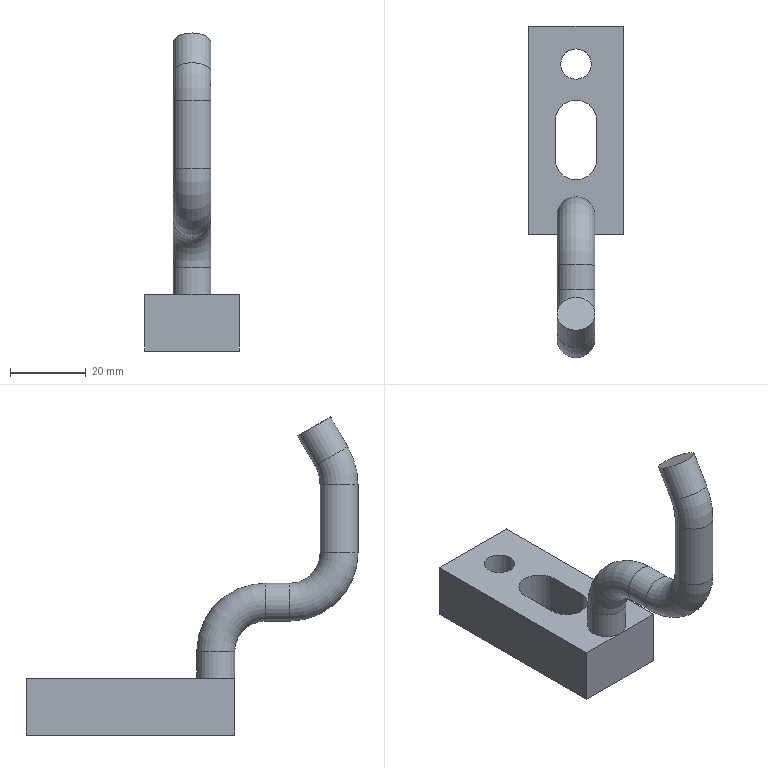Part | NX | features solid 2 | 1 solid | 19 faces | box 25 x 87.5 x 83.84 mm | volume 23805 mm3 | plane 9 | cylinder 7 | torus 3 | commonest cylinder face diameters 10 x4 11 x2 8 x1
STEP:
#1=CARTESIAN_POINT('',(-37.5,251.,-40.));
#2=VERTEX_POINT('',#1);
#3=CARTESIAN_POINT('',(-25.,251.,-40.));
#4=VERTEX_POINT('',#3);
#5=CARTESIAN_POINT('',(-37.,251.,-40.));
#6=DIRECTION('',(-1.,0.,0.));
#7=VECTOR('',#6,1000.);
#8=LINE('',#5,#7);
#9=EDGE_CURVE('',#2,#4,#8,.F.);
#10=ORIENTED_EDGE('',*,*,#9,.T.);
#11=CARTESIAN_POINT('',(-25.,256.,-40.));
#12=DIRECTION('',(0.,0.,1.));
#13=DIRECTION('',(0.,-1.,0.));
#14=AXIS2_PLACEMENT_3D('',#11,#12,#13);
#15=CIRCLE('',#14,5.);
#16=EDGE_CURVE('',#4,#4,#15,.T.);
#17=ORIENTED_EDGE('',*,*,#16,.F.);
#18=CARTESIAN_POINT('',(-12.5,251.,-40.));
#19=VERTEX_POINT('',#18);
#20=CARTESIAN_POINT('',(-37.,251.,-40.));
#21=DIRECTION('',(-1.,0.,0.));
#22=VECTOR('',#21,1000.);
#23=LINE('',#20,#22);
#24=EDGE_CURVE('',#4,#19,#23,.F.);
#25=ORIENTED_EDGE('',*,*,#24,.T.);
#26=CARTESIAN_POINT('',(-12.5,306.,-40.));
#27=VERTEX_POINT('',#26);
#28=CARTESIAN_POINT('',(-12.5,251.,-40.));
#29=DIRECTION('',(0.,1.,0.));
#30=VECTOR('',#29,1000.);
#31=LINE('',#28,#30);
#32=EDGE_CURVE('',#19,#27,#31,.T.);
#33=ORIENTED_EDGE('',*,*,#32,.T.);
#34=CARTESIAN_POINT('',(-37.5,306.,-40.));
#35=VERTEX_POINT('',#34);
#36=CARTESIAN_POINT('',(-37.,306.,-40.));
#37=DIRECTION('',(-1.,0.,0.));
#38=VECTOR('',#37,1000.);
#39=LINE('',#36,#38);
#40=EDGE_CURVE('',#27,#35,#39,.T.);
#41=ORIENTED_EDGE('',*,*,#40,.T.);
#42=CARTESIAN_POINT('',(-37.5,321.,-40.));
#43=DIRECTION('',(0.,-1.,0.));
#44=VECTOR('',#43,1000.);
#45=LINE('',#42,#44);
#46=EDGE_CURVE('',#35,#2,#45,.T.);
#47=ORIENTED_EDGE('',*,*,#46,.T.);
#48=EDGE_LOOP('',(#10,#17,#25,#33,#41,#47));
#49=FACE_BOUND('',#48,.T.);
#50=CARTESIAN_POINT('',(-30.5,271.,-40.));
#51=VERTEX_POINT('',#50);
#52=CARTESIAN_POINT('',(-30.5,281.,-40.));
#53=VERTEX_POINT('',#52);
#54=CARTESIAN_POINT('',(-30.5,281.,-40.));
#55=DIRECTION('',(0.,1.,0.));
#56=VECTOR('',#55,1000.);
#57=LINE('',#54,#56);
#58=EDGE_CURVE('',#51,#53,#57,.T.);
#59=ORIENTED_EDGE('',*,*,#58,.T.);
#60=CARTESIAN_POINT('',(-19.5,281.,-40.));
#61=VERTEX_POINT('',#60);
#62=CARTESIAN_POINT('',(-25.,281.,-40.));
#63=DIRECTION('',(0.,0.,1.));
#64=DIRECTION('',(0.,1.,0.));
#65=AXIS2_PLACEMENT_3D('',#62,#63,#64);
#66=CIRCLE('',#65,5.5);
#67=EDGE_CURVE('',#61,#53,#66,.T.);
#68=ORIENTED_EDGE('',*,*,#67,.F.);
#69=CARTESIAN_POINT('',(-19.5,271.,-40.));
#70=VERTEX_POINT('',#69);
#71=CARTESIAN_POINT('',(-19.5,286.,-40.));
#72=DIRECTION('',(0.,1.,0.));
#73=VECTOR('',#72,1000.);
#74=LINE('',#71,#73);
#75=EDGE_CURVE('',#70,#61,#74,.T.);
#76=ORIENTED_EDGE('',*,*,#75,.F.);
#77=CARTESIAN_POINT('',(-25.,271.,-40.));
#78=DIRECTION('',(0.,0.,1.));
#79=DIRECTION('',(0.,1.,0.));
#80=AXIS2_PLACEMENT_3D('',#77,#78,#79);
#81=CIRCLE('',#80,5.5);
#82=EDGE_CURVE('',#51,#70,#81,.T.);
#83=ORIENTED_EDGE('',*,*,#82,.F.);
#84=EDGE_LOOP('',(#59,#68,#76,#83));
#85=FACE_BOUND('',#84,.T.);
#86=CARTESIAN_POINT('',(-25.,292.,-40.));
#87=VERTEX_POINT('',#86);
#88=CARTESIAN_POINT('',(-25.,296.,-40.));
#89=DIRECTION('',(0.,0.,-1.));
#90=DIRECTION('',(0.,-1.,0.));
#91=AXIS2_PLACEMENT_3D('',#88,#89,#90);
#92=CIRCLE('',#91,4.);
#93=EDGE_CURVE('',#87,#87,#92,.T.);
#94=ORIENTED_EDGE('',*,*,#93,.T.);
#95=EDGE_LOOP('',(#94));
#96=FACE_BOUND('',#95,.T.);
#97=CARTESIAN_POINT('',(-37.,321.,-40.));
#98=DIRECTION('',(0.,0.,1.));
#99=DIRECTION('',(0.,-1.,0.));
#100=AXIS2_PLACEMENT_3D('',#97,#98,#99);
#101=PLANE('',#100);
#102=ADVANCED_FACE('',(#49,#85,#96),#101,.T.);
#103=CARTESIAN_POINT('',(-37.5,306.,-55.));
#104=VERTEX_POINT('',#103);
#105=CARTESIAN_POINT('',(-37.5,251.,-55.));
#106=VERTEX_POINT('',#105);
#107=CARTESIAN_POINT('',(-37.5,321.,-55.));
#108=DIRECTION('',(0.,-1.,0.));
#109=VECTOR('',#108,1000.);
#110=LINE('',#107,#109);
#111=EDGE_CURVE('',#104,#106,#110,.T.);
#112=ORIENTED_EDGE('',*,*,#111,.T.);
#113=CARTESIAN_POINT('',(-37.5,251.,-65.));
#114=DIRECTION('',(0.,0.,-1.));
#115=VECTOR('',#114,1000.);
#116=LINE('',#113,#115);
#117=EDGE_CURVE('',#2,#106,#116,.T.);
#118=ORIENTED_EDGE('',*,*,#117,.F.);
#119=ORIENTED_EDGE('',*,*,#46,.F.);
#120=CARTESIAN_POINT('',(-37.5,306.,-65.));
#121=DIRECTION('',(0.,0.,-1.));
#122=VECTOR('',#121,1000.);
#123=LINE('',#120,#122);
#124=EDGE_CURVE('',#35,#104,#123,.T.);
#125=ORIENTED_EDGE('',*,*,#124,.T.);
#126=EDGE_LOOP('',(#112,#118,#119,#125));
#127=FACE_BOUND('',#126,.T.);
#128=CARTESIAN_POINT('',(-37.5,321.,-65.));
#129=DIRECTION('',(1.,0.,0.));
#130=DIRECTION('',(0.,1.,0.));
#131=AXIS2_PLACEMENT_3D('',#128,#129,#130);
#132=PLANE('',#131);
#133=ADVANCED_FACE('',(#127),#132,.F.);
#134=CARTESIAN_POINT('',(-12.5,306.,-55.));
#135=VERTEX_POINT('',#134);
#136=CARTESIAN_POINT('',(-37.,306.,-55.));
#137=DIRECTION('',(-1.,0.,0.));
#138=VECTOR('',#137,1000.);
#139=LINE('',#136,#138);
#140=EDGE_CURVE('',#135,#104,#139,.T.);
#141=ORIENTED_EDGE('',*,*,#140,.T.);
#142=ORIENTED_EDGE('',*,*,#124,.F.);
#143=ORIENTED_EDGE('',*,*,#40,.F.);
#144=CARTESIAN_POINT('',(-12.5,306.,-40.));
#145=DIRECTION('',(0.,0.,-1.));
#146=VECTOR('',#145,1000.);
#147=LINE('',#144,#146);
#148=EDGE_CURVE('',#27,#135,#147,.T.);
#149=ORIENTED_EDGE('',*,*,#148,.T.);
#150=EDGE_LOOP('',(#141,#142,#143,#149));
#151=FACE_BOUND('',#150,.T.);
#152=CARTESIAN_POINT('',(-13.,306.,-65.));
#153=DIRECTION('',(0.,-1.,0.));
#154=DIRECTION('',(0.,0.,1.));
#155=AXIS2_PLACEMENT_3D('',#152,#153,#154);
#156=PLANE('',#155);
#157=ADVANCED_FACE('',(#151),#156,.F.);
#158=CARTESIAN_POINT('',(-12.5,251.,-55.));
#159=VERTEX_POINT('',#158);
#160=CARTESIAN_POINT('',(-12.5,321.,-55.));
#161=DIRECTION('',(0.,1.,0.));
#162=VECTOR('',#161,1000.);
#163=LINE('',#160,#162);
#164=EDGE_CURVE('',#159,#135,#163,.T.);
#165=ORIENTED_EDGE('',*,*,#164,.T.);
#166=ORIENTED_EDGE('',*,*,#148,.F.);
#167=ORIENTED_EDGE('',*,*,#32,.F.);
#168=CARTESIAN_POINT('',(-12.5,251.,-40.));
#169=DIRECTION('',(0.,0.,-1.));
#170=VECTOR('',#169,1000.);
#171=LINE('',#168,#170);
#172=EDGE_CURVE('',#19,#159,#171,.T.);
#173=ORIENTED_EDGE('',*,*,#172,.T.);
#174=EDGE_LOOP('',(#165,#166,#167,#173));
#175=FACE_BOUND('',#174,.T.);
#176=CARTESIAN_POINT('',(-12.5,251.,-40.));
#177=DIRECTION('',(-1.,0.,0.));
#178=DIRECTION('',(0.,-1.,0.));
#179=AXIS2_PLACEMENT_3D('',#176,#177,#178);
#180=PLANE('',#179);
#181=ADVANCED_FACE('',(#175),#180,.F.);
#182=ORIENTED_EDGE('',*,*,#93,.F.);
#183=EDGE_LOOP('',(#182));
#184=FACE_BOUND('',#183,.T.);
#185=CARTESIAN_POINT('',(-25.,292.,-55.));
#186=VERTEX_POINT('',#185);
#187=CARTESIAN_POINT('',(-25.,296.,-55.));
#188=DIRECTION('',(0.,0.,-1.));
#189=DIRECTION('',(0.,-1.,0.));
#190=AXIS2_PLACEMENT_3D('',#187,#188,#189);
#191=CIRCLE('',#190,4.);
#192=EDGE_CURVE('',#186,#186,#191,.F.);
#193=ORIENTED_EDGE('',*,*,#192,.F.);
#194=EDGE_LOOP('',(#193));
#195=FACE_BOUND('',#194,.T.);
#196=CARTESIAN_POINT('',(-25.,296.,-65.));
#197=DIRECTION('',(0.,0.,-1.));
#198=DIRECTION('',(0.,-1.,0.));
#199=AXIS2_PLACEMENT_3D('',#196,#197,#198);
#200=CYLINDRICAL_SURFACE('',#199,4.);
#201=ADVANCED_FACE('',(#184,#195),#200,.F.);
#202=ORIENTED_EDGE('',*,*,#82,.T.);
#203=CARTESIAN_POINT('',(-19.5,271.,-55.));
#204=VERTEX_POINT('',#203);
#205=CARTESIAN_POINT('',(-19.5,271.,-65.));
#206=DIRECTION('',(0.,0.,1.));
#207=VECTOR('',#206,1000.);
#208=LINE('',#205,#207);
#209=EDGE_CURVE('',#204,#70,#208,.T.);
#210=ORIENTED_EDGE('',*,*,#209,.F.);
#211=CARTESIAN_POINT('',(-30.5,271.,-55.));
#212=VERTEX_POINT('',#211);
#213=CARTESIAN_POINT('',(-25.,271.,-55.));
#214=DIRECTION('',(0.,0.,-1.));
#215=DIRECTION('',(0.,-1.,0.));
#216=AXIS2_PLACEMENT_3D('',#213,#214,#215);
#217=CIRCLE('',#216,5.5);
#218=EDGE_CURVE('',#212,#204,#217,.F.);
#219=ORIENTED_EDGE('',*,*,#218,.F.);
#220=CARTESIAN_POINT('',(-30.5,271.,-65.));
#221=DIRECTION('',(0.,0.,1.));
#222=VECTOR('',#221,1000.);
#223=LINE('',#220,#222);
#224=EDGE_CURVE('',#212,#51,#223,.T.);
#225=ORIENTED_EDGE('',*,*,#224,.T.);
#226=EDGE_LOOP('',(#202,#210,#219,#225));
#227=FACE_BOUND('',#226,.T.);
#228=CARTESIAN_POINT('',(-25.,271.,-65.));
#229=DIRECTION('',(0.,0.,1.));
#230=DIRECTION('',(0.,1.,0.));
#231=AXIS2_PLACEMENT_3D('',#228,#229,#230);
#232=CYLINDRICAL_SURFACE('',#231,5.5);
#233=ADVANCED_FACE('',(#227),#232,.F.);
#234=ORIENTED_EDGE('',*,*,#75,.T.);
#235=CARTESIAN_POINT('',(-19.5,281.,-55.));
#236=VERTEX_POINT('',#235);
#237=CARTESIAN_POINT('',(-19.5,281.,-65.));
#238=DIRECTION('',(0.,0.,1.));
#239=VECTOR('',#238,1000.);
#240=LINE('',#237,#239);
#241=EDGE_CURVE('',#236,#61,#240,.T.);
#242=ORIENTED_EDGE('',*,*,#241,.F.);
#243=CARTESIAN_POINT('',(-19.5,286.,-55.));
#244=DIRECTION('',(0.,1.,0.));
#245=VECTOR('',#244,1000.);
#246=LINE('',#243,#245);
#247=EDGE_CURVE('',#204,#236,#246,.T.);
#248=ORIENTED_EDGE('',*,*,#247,.F.);
#249=ORIENTED_EDGE('',*,*,#209,.T.);
#250=EDGE_LOOP('',(#234,#242,#248,#249));
#251=FACE_BOUND('',#250,.T.);
#252=CARTESIAN_POINT('',(-19.5,286.,-65.));
#253=DIRECTION('',(1.,0.,0.));
#254=DIRECTION('',(0.,0.,-1.));
#255=AXIS2_PLACEMENT_3D('',#252,#253,#254);
#256=PLANE('',#255);
#257=ADVANCED_FACE('',(#251),#256,.F.);
#258=ORIENTED_EDGE('',*,*,#67,.T.);
#259=CARTESIAN_POINT('',(-30.5,281.,-55.));
#260=VERTEX_POINT('',#259);
#261=CARTESIAN_POINT('',(-30.5,281.,-65.));
#262=DIRECTION('',(0.,0.,1.));
#263=VECTOR('',#262,1000.);
#264=LINE('',#261,#263);
#265=EDGE_CURVE('',#260,#53,#264,.T.);
#266=ORIENTED_EDGE('',*,*,#265,.F.);
#267=CARTESIAN_POINT('',(-25.,281.,-55.));
#268=DIRECTION('',(0.,0.,-1.));
#269=DIRECTION('',(0.,-1.,0.));
#270=AXIS2_PLACEMENT_3D('',#267,#268,#269);
#271=CIRCLE('',#270,5.5);
#272=EDGE_CURVE('',#236,#260,#271,.F.);
#273=ORIENTED_EDGE('',*,*,#272,.F.);
#274=ORIENTED_EDGE('',*,*,#241,.T.);
#275=EDGE_LOOP('',(#258,#266,#273,#274));
#276=FACE_BOUND('',#275,.T.);
#277=CARTESIAN_POINT('',(-25.,281.,-65.));
#278=DIRECTION('',(0.,0.,1.));
#279=DIRECTION('',(0.,1.,0.));
#280=AXIS2_PLACEMENT_3D('',#277,#278,#279);
#281=CYLINDRICAL_SURFACE('',#280,5.5);
#282=ADVANCED_FACE('',(#276),#281,.F.);
#283=ORIENTED_EDGE('',*,*,#58,.F.);
#284=ORIENTED_EDGE('',*,*,#224,.F.);
#285=CARTESIAN_POINT('',(-30.5,321.,-55.));
#286=DIRECTION('',(0.,1.,0.));
#287=VECTOR('',#286,1000.);
#288=LINE('',#285,#287);
#289=EDGE_CURVE('',#212,#260,#288,.T.);
#290=ORIENTED_EDGE('',*,*,#289,.T.);
#291=ORIENTED_EDGE('',*,*,#265,.T.);
#292=EDGE_LOOP('',(#283,#284,#290,#291));
#293=FACE_BOUND('',#292,.T.);
#294=CARTESIAN_POINT('',(-30.5,281.,-65.));
#295=DIRECTION('',(-1.,0.,0.));
#296=DIRECTION('',(0.,0.,1.));
#297=AXIS2_PLACEMENT_3D('',#294,#295,#296);
#298=PLANE('',#297);
#299=ADVANCED_FACE('',(#293),#298,.F.);
#300=CARTESIAN_POINT('',(-37.,251.,-55.));
#301=DIRECTION('',(1.,0.,0.));
#302=VECTOR('',#301,1000.);
#303=LINE('',#300,#302);
#304=EDGE_CURVE('',#106,#159,#303,.T.);
#305=ORIENTED_EDGE('',*,*,#304,.F.);
#306=ORIENTED_EDGE('',*,*,#111,.F.);
#307=ORIENTED_EDGE('',*,*,#140,.F.);
#308=ORIENTED_EDGE('',*,*,#164,.F.);
#309=EDGE_LOOP('',(#305,#306,#307,#308));
#310=FACE_BOUND('',#309,.T.);
#311=ORIENTED_EDGE('',*,*,#272,.T.);
#312=ORIENTED_EDGE('',*,*,#289,.F.);
#313=ORIENTED_EDGE('',*,*,#218,.T.);
#314=ORIENTED_EDGE('',*,*,#247,.T.);
#315=EDGE_LOOP('',(#311,#312,#313,#314));
#316=FACE_BOUND('',#315,.T.);
#317=ORIENTED_EDGE('',*,*,#192,.T.);
#318=EDGE_LOOP('',(#317));
#319=FACE_BOUND('',#318,.T.);
#320=CARTESIAN_POINT('',(-37.,321.,-55.));
#321=DIRECTION('',(0.,0.,1.));
#322=DIRECTION('',(0.,1.,0.));
#323=AXIS2_PLACEMENT_3D('',#320,#321,#322);
#324=PLANE('',#323);
#325=ADVANCED_FACE('',(#310,#316,#319),#324,.F.);
#326=ORIENTED_EDGE('',*,*,#117,.T.);
#327=ORIENTED_EDGE('',*,*,#304,.T.);
#328=ORIENTED_EDGE('',*,*,#172,.F.);
#329=ORIENTED_EDGE('',*,*,#24,.F.);
#330=ORIENTED_EDGE('',*,*,#9,.F.);
#331=EDGE_LOOP('',(#326,#327,#328,#329,#330));
#332=FACE_BOUND('',#331,.T.);
#333=CARTESIAN_POINT('',(-37.,251.,-65.));
#334=DIRECTION('',(0.,1.,0.));
#335=DIRECTION('',(0.,0.,-1.));
#336=AXIS2_PLACEMENT_3D('',#333,#334,#335);
#337=PLANE('',#336);
#338=ADVANCED_FACE('',(#332),#337,.F.);
#339=ORIENTED_EDGE('',*,*,#16,.T.);
#340=EDGE_LOOP('',(#339));
#341=FACE_BOUND('',#340,.T.);
#342=CARTESIAN_POINT('',(-25.,251.,-33.));
#343=VERTEX_POINT('',#342);
#344=CARTESIAN_POINT('',(-25.,256.,-33.));
#345=DIRECTION('',(0.,0.,1.));
#346=DIRECTION('',(0.,-1.,0.));
#347=AXIS2_PLACEMENT_3D('',#344,#345,#346);
#348=CIRCLE('',#347,5.);
#349=EDGE_CURVE('',#343,#343,#348,.T.);
#350=ORIENTED_EDGE('',*,*,#349,.F.);
#351=EDGE_LOOP('',(#350));
#352=FACE_BOUND('',#351,.T.);
#353=CARTESIAN_POINT('',(-25.,256.,-65.));
#354=DIRECTION('',(0.,0.,1.));
#355=DIRECTION('',(0.,-1.,0.));
#356=AXIS2_PLACEMENT_3D('',#353,#354,#355);
#357=CYLINDRICAL_SURFACE('',#356,5.);
#358=ADVANCED_FACE('',(#341,#352),#357,.T.);
#359=CARTESIAN_POINT('',(-25.,218.5,-7.));
#360=VERTEX_POINT('',#359);
#361=CARTESIAN_POINT('',(-25.,223.5,-7.));
#362=DIRECTION('',(0.,0.,1.));
#363=DIRECTION('',(0.,-1.,0.));
#364=AXIS2_PLACEMENT_3D('',#361,#362,#363);
#365=CIRCLE('',#364,5.);
#366=EDGE_CURVE('',#360,#360,#365,.T.);
#367=ORIENTED_EDGE('',*,*,#366,.T.);
#368=EDGE_LOOP('',(#367));
#369=FACE_BOUND('',#368,.T.);
#370=CARTESIAN_POINT('',(-25.,228.5,10.981));
#371=VERTEX_POINT('',#370);
#372=CARTESIAN_POINT('',(-25.,223.5,10.981));
#373=DIRECTION('',(0.,0.,-1.));
#374=DIRECTION('',(0.,1.,0.));
#375=AXIS2_PLACEMENT_3D('',#372,#373,#374);
#376=CIRCLE('',#375,5.);
#377=EDGE_CURVE('',#371,#371,#376,.F.);
#378=ORIENTED_EDGE('',*,*,#377,.F.);
#379=EDGE_LOOP('',(#378));
#380=FACE_BOUND('',#379,.T.);
#381=CARTESIAN_POINT('',(-25.,223.5,-7.));
#382=DIRECTION('',(0.,0.,1.));
#383=DIRECTION('',(-1.,0.,0.));
#384=AXIS2_PLACEMENT_3D('',#381,#382,#383);
#385=CYLINDRICAL_SURFACE('',#384,5.);
#386=ADVANCED_FACE('',(#369,#380),#385,.T.);
#387=CARTESIAN_POINT('',(-25.,236.5,-25.));
#388=VERTEX_POINT('',#387);
#389=CARTESIAN_POINT('',(-25.,236.5,-20.));
#390=DIRECTION('',(0.,-1.,0.));
#391=DIRECTION('',(0.,0.,-1.));
#392=AXIS2_PLACEMENT_3D('',#389,#390,#391);
#393=CIRCLE('',#392,5.);
#394=EDGE_CURVE('',#388,#388,#393,.T.);
#395=ORIENTED_EDGE('',*,*,#394,.T.);
#396=EDGE_LOOP('',(#395));
#397=FACE_BOUND('',#396,.T.);
#398=ORIENTED_EDGE('',*,*,#366,.F.);
#399=EDGE_LOOP('',(#398));
#400=FACE_BOUND('',#399,.T.);
#401=CARTESIAN_POINT('',(-25.,236.5,-7.));
#402=DIRECTION('',(-1.,0.,0.));
#403=DIRECTION('',(0.,0.,-1.));
#404=AXIS2_PLACEMENT_3D('',#401,#402,#403);
#405=TOROIDAL_SURFACE('',#404,13.,5.);
#406=ADVANCED_FACE('',(#397,#400),#405,.T.);
#407=CARTESIAN_POINT('',(-25.,243.,-25.));
#408=VERTEX_POINT('',#407);
#409=CARTESIAN_POINT('',(-25.,243.,-20.));
#410=DIRECTION('',(0.,-1.,0.));
#411=DIRECTION('',(0.,0.,-1.));
#412=AXIS2_PLACEMENT_3D('',#409,#410,#411);
#413=CIRCLE('',#412,5.);
#414=EDGE_CURVE('',#408,#408,#413,.T.);
#415=ORIENTED_EDGE('',*,*,#414,.T.);
#416=EDGE_LOOP('',(#415));
#417=FACE_BOUND('',#416,.T.);
#418=ORIENTED_EDGE('',*,*,#394,.F.);
#419=EDGE_LOOP('',(#418));
#420=FACE_BOUND('',#419,.T.);
#421=CARTESIAN_POINT('',(-25.,243.,-20.));
#422=DIRECTION('',(0.,-1.,0.));
#423=DIRECTION('',(0.,0.,-1.));
#424=AXIS2_PLACEMENT_3D('',#421,#422,#423);
#425=CYLINDRICAL_SURFACE('',#424,5.);
#426=ADVANCED_FACE('',(#417,#420),#425,.T.);
#427=ORIENTED_EDGE('',*,*,#349,.T.);
#428=EDGE_LOOP('',(#427));
#429=FACE_BOUND('',#428,.T.);
#430=ORIENTED_EDGE('',*,*,#414,.F.);
#431=EDGE_LOOP('',(#430));
#432=FACE_BOUND('',#431,.T.);
#433=CARTESIAN_POINT('',(-25.,243.,-33.));
#434=DIRECTION('',(1.,0.,0.));
#435=DIRECTION('',(0.,0.,1.));
#436=AXIS2_PLACEMENT_3D('',#433,#434,#435);
#437=TOROIDAL_SURFACE('',#436,13.,5.);
#438=ADVANCED_FACE('',(#429,#432),#437,.T.);
#439=CARTESIAN_POINT('',(-25.,221.179,20.981));
#440=VERTEX_POINT('',#439);
#441=CARTESIAN_POINT('',(-25.,225.51,18.481));
#442=DIRECTION('',(0.,0.5,0.866));
#443=DIRECTION('',(0.,-0.866,0.5));
#444=AXIS2_PLACEMENT_3D('',#441,#442,#443);
#445=CIRCLE('',#444,5.);
#446=EDGE_CURVE('',#440,#440,#445,.T.);
#447=ORIENTED_EDGE('',*,*,#446,.T.);
#448=EDGE_LOOP('',(#447));
#449=FACE_BOUND('',#448,.T.);
#450=CARTESIAN_POINT('',(-25.,225.717,28.84));
#451=VERTEX_POINT('',#450);
#452=CARTESIAN_POINT('',(-25.,230.047,26.34));
#453=DIRECTION('',(0.,0.5,0.866));
#454=DIRECTION('',(0.,-0.866,0.5));
#455=AXIS2_PLACEMENT_3D('',#452,#453,#454);
#456=CIRCLE('',#455,5.);
#457=EDGE_CURVE('',#451,#451,#456,.T.);
#458=ORIENTED_EDGE('',*,*,#457,.F.);
#459=EDGE_LOOP('',(#458));
#460=FACE_BOUND('',#459,.T.);
#461=CARTESIAN_POINT('',(-25.,225.51,18.481));
#462=DIRECTION('',(0.,0.5,0.866));
#463=DIRECTION('',(0.,0.866,-0.5));
#464=AXIS2_PLACEMENT_3D('',#461,#462,#463);
#465=CYLINDRICAL_SURFACE('',#464,5.);
#466=ADVANCED_FACE('',(#449,#460),#465,.T.);
#467=ORIENTED_EDGE('',*,*,#377,.T.);
#468=EDGE_LOOP('',(#467));
#469=FACE_BOUND('',#468,.T.);
#470=ORIENTED_EDGE('',*,*,#446,.F.);
#471=EDGE_LOOP('',(#470));
#472=FACE_BOUND('',#471,.T.);
#473=CARTESIAN_POINT('',(-25.,238.5,10.981));
#474=DIRECTION('',(-1.,0.,0.));
#475=DIRECTION('',(0.,0.,1.));
#476=AXIS2_PLACEMENT_3D('',#473,#474,#475);
#477=TOROIDAL_SURFACE('',#476,15.,5.);
#478=ADVANCED_FACE('',(#469,#472),#477,.T.);
#479=ORIENTED_EDGE('',*,*,#457,.T.);
#480=EDGE_LOOP('',(#479));
#481=FACE_BOUND('',#480,.T.);
#482=CARTESIAN_POINT('',(-25.,230.047,26.34));
#483=DIRECTION('',(0.,0.5,0.866));
#484=DIRECTION('',(0.,0.866,-0.5));
#485=AXIS2_PLACEMENT_3D('',#482,#483,#484);
#486=PLANE('',#485);
#487=ADVANCED_FACE('',(#481),#486,.T.);
#488=CLOSED_SHELL('',(#102,#133,#157,#181,#201,#233,#257,#282,#299,#325,#338,#358,#386,#406,#426,#438,#466,#478,#487));
#489=MANIFOLD_SOLID_BREP('',#488);
#490=(LENGTH_UNIT()NAMED_UNIT(*)SI_UNIT(.MILLI.,.METRE.));
#491=UNCERTAINTY_MEASURE_WITH_UNIT(LENGTH_MEASURE(0.00001),#490,'','');
#492=(NAMED_UNIT(*)PLANE_ANGLE_UNIT()SI_UNIT($,.RADIAN.));
#493=(NAMED_UNIT(*)SI_UNIT($,.STERADIAN.)SOLID_ANGLE_UNIT());
#494=(GEOMETRIC_REPRESENTATION_CONTEXT(3)GLOBAL_UNCERTAINTY_ASSIGNED_CONTEXT((#491))GLOBAL_UNIT_ASSIGNED_CONTEXT((#490,#492,#493))REPRESENTATION_CONTEXT('',''));
#495=ADVANCED_BREP_SHAPE_REPRESENTATION('',(#489),#494);